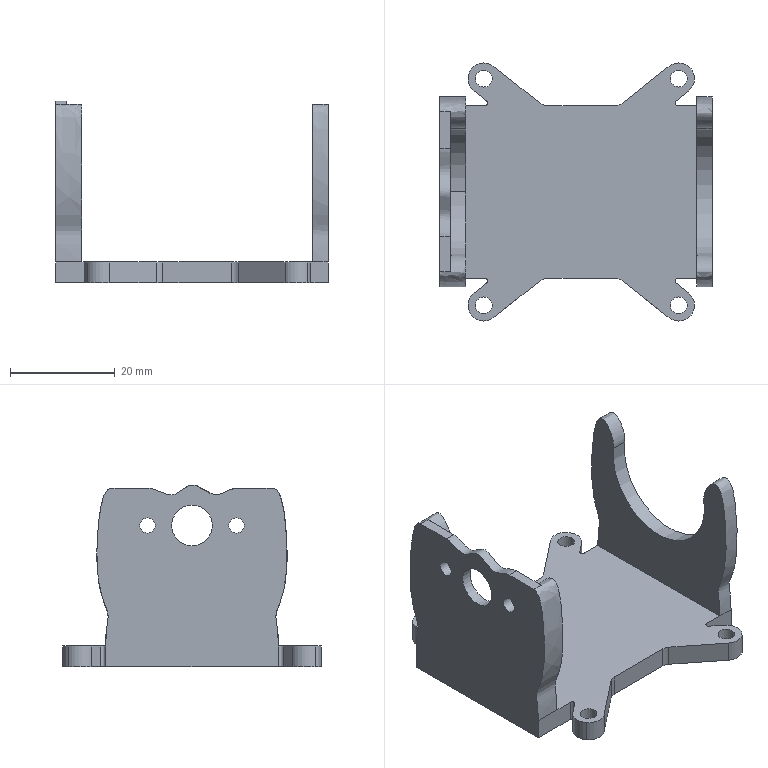Part | STEP file | Dodanie-wyci_gni_cie4 | 1 solid | 56 faces | box 52 x 49.249 x 34.708 mm | volume 13507 mm3 | cylinder 28 | plane 23 | spline 5 | commonest cylinder face diameters 5.998 x10 1 x4 3.2 x4 4 x4 24.6 x3 2.9 x2